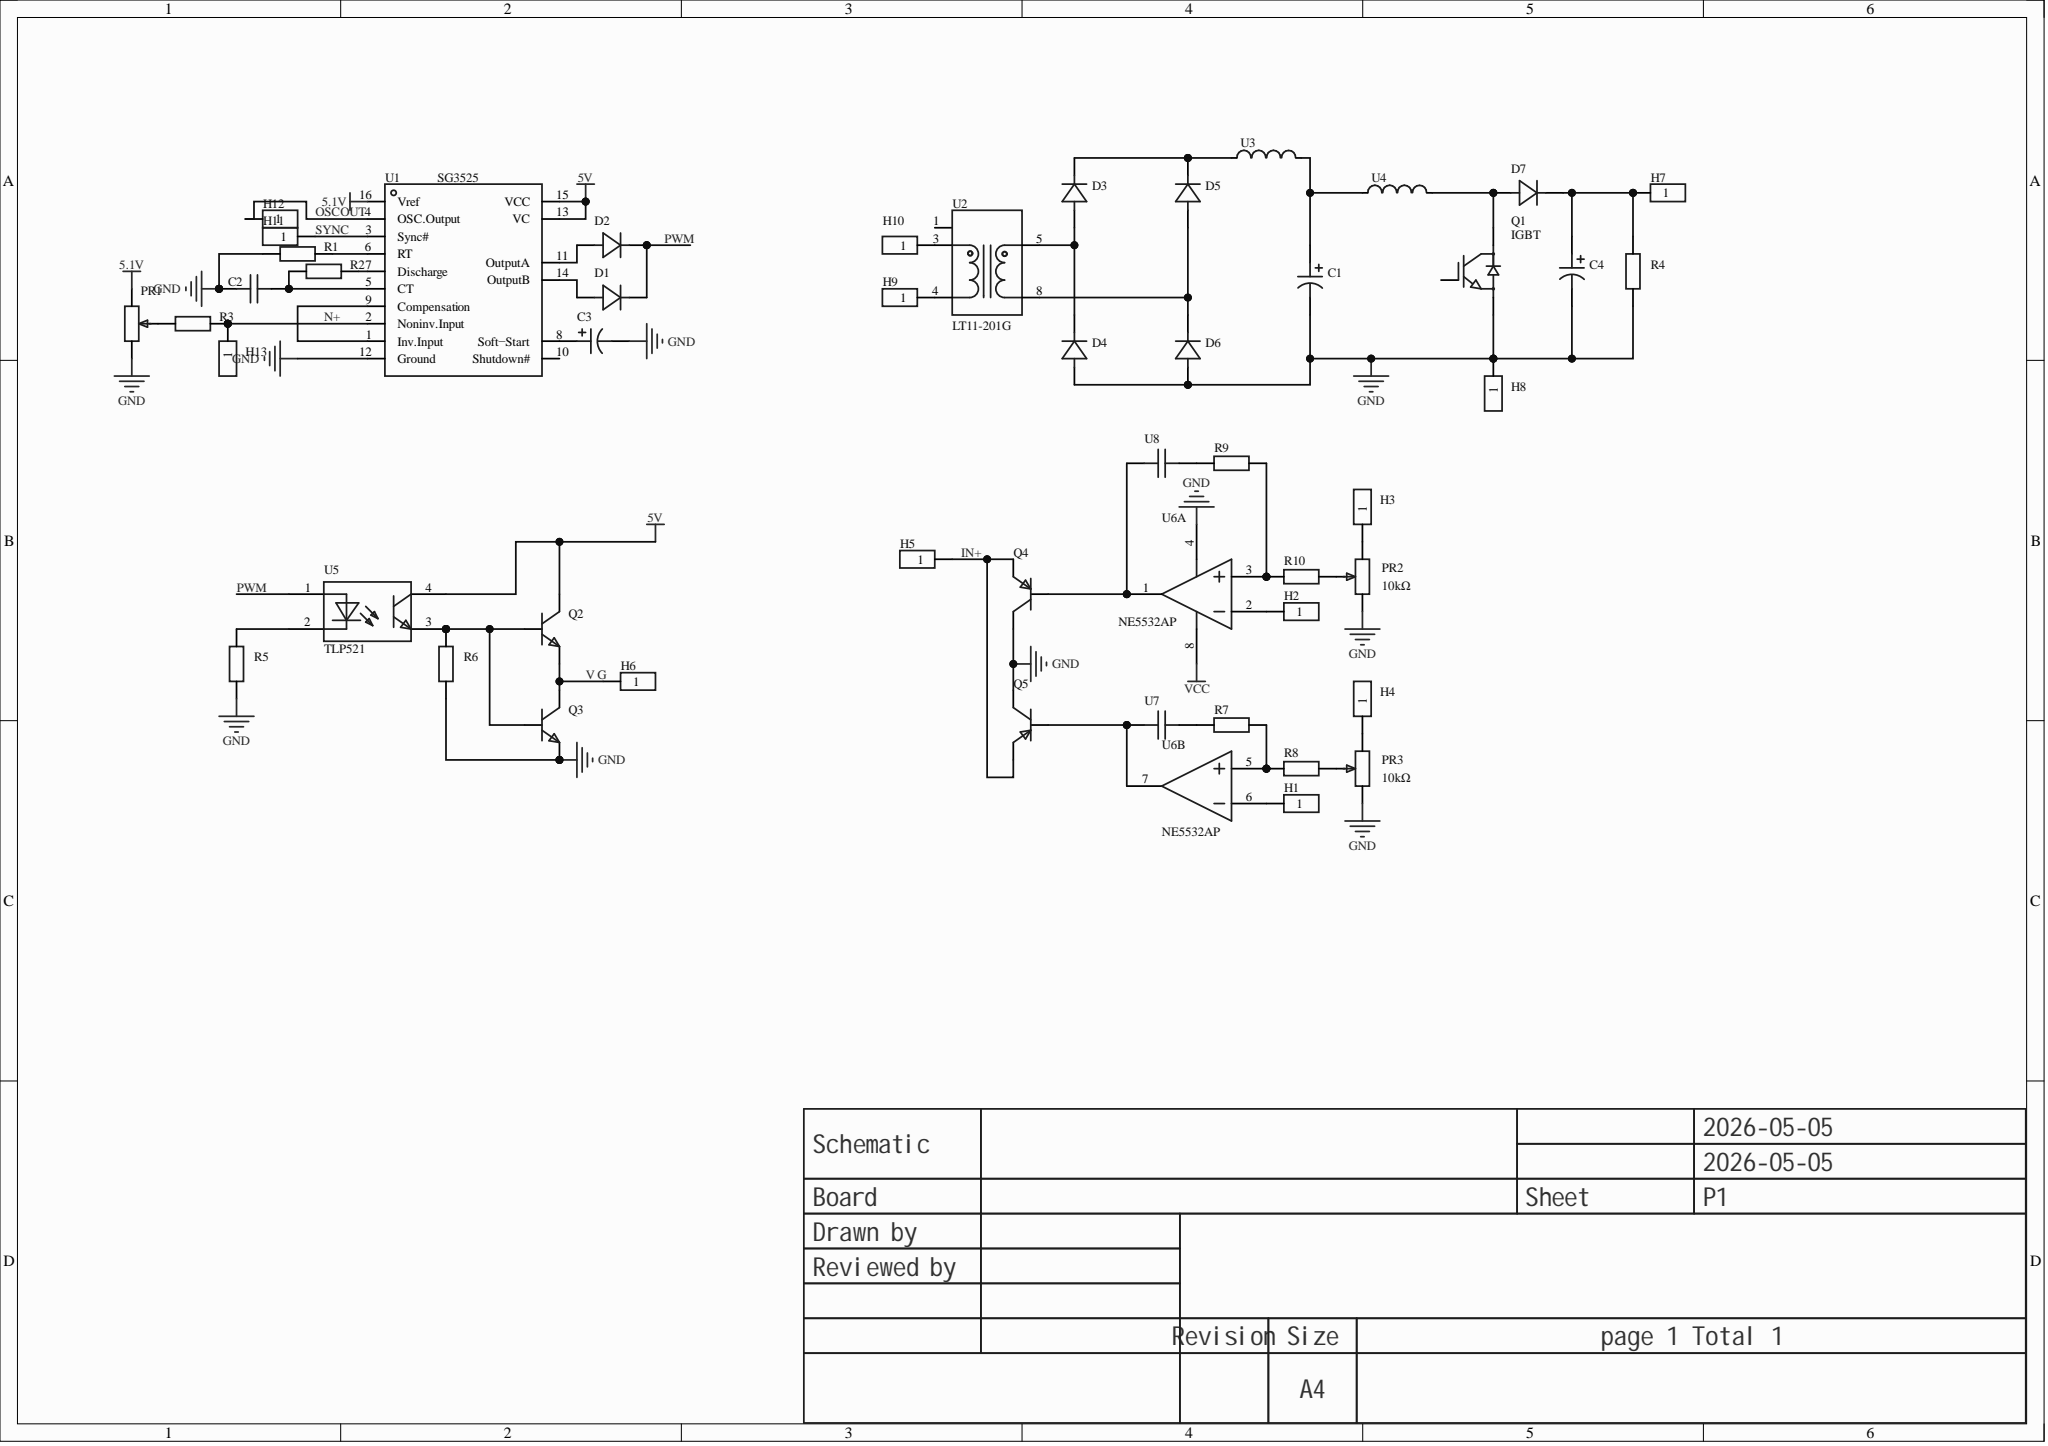Circuit board | Altium Designer | 50 parts | 39 nets
Bill of materials:
Comment,Description,Designator,Footprint,LibRef,Quantity
"10uF","Capacitance:10uF;Tolerance:±20%;Rated voltage:50V;Ripple current:120mA@100KHz;Equivalent series resistance(ESR):1.6Ω;","C1, C3, C4","CAP-TH_BD5.0-P2.00-D0.8-FD-10UF50VC110GL","10UF50VC110GL","3"
"100nF","","C2, U7, U8","CAP-TH_L5.0-W2.5-P5.00-D1.0","100nF","3"
"","","D1, D2, D3, D4, D5, D6, D7","DO_1N4007","D_1N4007A","7"
"","","H1, H2, H3, H4, H5, H6, H7, H8, H9, H10, H11, H12, H13","HDR-TH_1P-V-M_XKB_X4611WV-01I-C28D40","HDR-M_2.54_1x1P","13"
"10kΩ","","PR1, PR2, PR3","R_3296","R_3296","3"
"IGBT","Uses advanced trench gate field-stop technology (Trench FS), collector-emitter breakdown voltage Vces=650V, collector current Ic=40A, with low conduction voltage drop and low turn-off loss, etc…","Q1","TO-247-3_L15.9-W5.0-P5.44-L","MLG40T65FDL-W","1"
"","","Q2, Q3","S8050_TO_92","S8050_TO_NPN","2"
"","","Q4, Q5","S8550P_SOT","S8550_SOT_PNP","2"
"10kΩ","","R1, R2, R3, R4, R5, R6, R7, R8, R9, R10","Res_1/8W","Res_AXIAL-1/8W","10"
"SG3525","Operating voltage: 8V~35V; switching frequency: 100Hz~500kHz; output current: 400mA; transistor withstand voltage: -;","U1","DIP-16_L19.2-W6.6-P2.54-LS7.6-BL","SG3525","1"
"LT11-201G","Transformer  Through-hole broadband carrier coupling transformer, high withstand voltage","U2","XFMR-TH_LT13-201","LT11-201G","1"
"Power inductor (SMD), CKST0502-10uH/M, 10uH, ±20%, 3A, package 5.7mm*5.1mm*2.0mm, Cenke, RoHS","","U3, U4","IND-SMD_L5.7-W5.1","功率电感(贴片),CKST0502-10uH/M,10uH,±20%,3A,封装5.7mm*5.1mm*2.0mm,岑科,RoHS","2"
"TLP521","","U5","SOP-4_L6.4-W4.6-P2.54-LS10.2-TL","TLP521","1"
"NE5532AP","Dual-channel, 30V, 10MHz, low-noise (6nV/vHz) operational amplifier for audio applications","U6","PDIP-8_L9.6-W6.4-P2.54-LS7.6-BL","NE5532AP","1"
Netlist (Protel format):
[
C1
CAP-TH_BD5.0-P2.00-D0.8-FD-10UF50VC110GL
10uF



]
[
C2
CAP-TH_L5.0-W2.5-P5.00-D1.0
100nF



]
[
C3
CAP-TH_BD5.0-P2.00-D0.8-FD-10UF50VC110GL
10uF



]
[
C4
CAP-TH_BD5.0-P2.00-D0.8-FD-10UF50VC110GL
10uF



]
[
D1
DO_1N4007




]
[
D2
DO_1N4007




]
[
D3
DO_1N4007




]
[
D4
DO_1N4007




]
[
D5
DO_1N4007




]
[
D6
DO_1N4007




]
[
D7
DO_1N4007




]
[
H1
HDR-TH_1P-V-M_XKB_X4611WV-01I-C28D40




]
[
H2
HDR-TH_1P-V-M_XKB_X4611WV-01I-C28D40




]
[
H3
HDR-TH_1P-V-M_XKB_X4611WV-01I-C28D40




]
[
H4
HDR-TH_1P-V-M_XKB_X4611WV-01I-C28D40




]
[
H5
HDR-TH_1P-V-M_XKB_X4611WV-01I-C28D40




]
[
H6
HDR-TH_1P-V-M_XKB_X4611WV-01I-C28D40




]
[
H7
HDR-TH_1P-V-M_XKB_X4611WV-01I-C28D40




]
[
H8
HDR-TH_1P-V-M_XKB_X4611WV-01I-C28D40




]
[
H9
HDR-TH_1P-V-M_XKB_X4611WV-01I-C28D40




]
[
H10
HDR-TH_1P-V-M_XKB_X4611WV-01I-C28D40




]
[
H11
HDR-TH_1P-V-M_XKB_X4611WV-01I-C28D40




]
[
H12
HDR-TH_1P-V-M_XKB_X4611WV-01I-C28D40




]
[
H13
HDR-TH_1P-V-M_XKB_X4611WV-01I-C28D40




]
[
PR1
R_3296
10kΩ



]
[
PR2
R_3296
10kΩ



]
[
PR3
R_3296
10kΩ



]
[
Q1
TO-247-3_L15.9-W5.0-P5.44-L
IGBT



]
[
Q2
S8050_TO_92




]
[
Q3
S8050_TO_92




]
[
Q4
S8550P_SOT




]
[
Q5
S8550P_SOT




]
[
R1
Res_1/8W
10kΩ



]
[
R2
Res_1/8W
10kΩ



]
[
R3
Res_1/8W
10kΩ



]
[
R4
Res_1/8W
10kΩ



]
[
R5
Res_1/8W
10kΩ



]
[
R6
Res_1/8W
10kΩ



]
[
R7
Res_1/8W
10kΩ



]
[
R8
Res_1/8W
10kΩ



]
[
R9
Res_1/8W
10kΩ



]
[
R10
Res_1/8W
10kΩ



]
[
U1
DIP-16_L19.2-W6.6-P2.54-LS7.6-BL
SG3525



]
[
U2
XFMR-TH_LT13-201
LT11-201G



]
[
U3
IND-SMD_L5.7-W5.1
Power inductor (SMD), CKST0502-10uH/M, 10uH, ±20%, 3A, package 5.7mm*5.1mm*2.0mm, Cenke, RoHS



]
[
U4
IND-SMD_L5.7-W5.1
Power inductor (SMD), CKST0502-10uH/M, 10uH, ±20%, 3A, package 5.7mm*5.1mm*2.0mm, Cenke, RoHS



]
[
U5
SOP-4_L6.4-W4.6-P2.54-LS10.2-TL
TLP521



]
[
U6
PDIP-8_L9.6-W6.4-P2.54-LS7.6-BL
NE5532AP



]
[
U7
CAP-TH_L5.0-W2.5-P5.00-D1.0
100nF



]
[
U8
CAP-TH_L5.0-W2.5-P5.00-D1.0
100nF



]
(
V G
H6-1
Q2-1
Q3-3
)
(
SYNC
H11-1
U1-3
)
(
PWM
D1-1
D2-1
U5-1
)
(
OSCOUT
H12-1
U1-4
)
(
NetU1_1
U1-1
U1-9
)
(
NetR9_2
R9-2
U8-1
)
(
NetR9_1
R9-1
R10-2
U6-3
)
(
NetR7_2
R7-2
U7-1
)
(
NetR7_1
R7-1
R8-2
U6-5
)
(
NetR5_2
R5-2
U5-2
)
(
NetR2_2
R2-2
U1-7
)
(
NetR1_2
R1-2
U1-6
)
(
NetQ5_1
Q5-1
U6-7
U7-2
)
(
NetQ4_1
Q4-1
U6-1
U8-2
)
(
NetQ2_2
Q2-2
Q3-2
R6-2
U5-3
)
(
NetPR3_2
PR3-2
R8-1
)
(
NetPR2_2
PR2-2
R10-1
)
(
NetPR1_2
PR1-2
R3-1
)
(
NetH10_1
H10-1
U2-3
)
(
NetH9_1
H9-1
U2-4
)
(
NetH4_1
H4-1
PR3-1
)
(
NetH3_1
H3-1
PR2-1
)
(
NetH2_1
H2-1
U6-2
)
(
NetH1_1
H1-1
U6-6
)
(
NetD7_2
D7-2
Q1-2
U4-2
)
(
NetD5_2
D5-2
D6-1
U2-8
)
(
NetD3_2
D3-2
D4-1
U2-5
)
(
NetD3_1
D3-1
D5-1
U3-1
)
(
NetD2_2
D2-2
U1-11
)
(
NetD1_2
D1-2
U1-14
)
(
NetC4_1
C4-1
D7-1
H7-1
R4-2
)
(
NetC3_1
C3-1
U1-8
)
(
NetC2_1
C2-1
R2-1
U1-5
)
(
NetC1_1
C1-1
U3-2
U4-1
)
(
N+
H13-1
R3-2
U1-2
)
(
IN+
H5-1
Q4-2
Q5-2
)
(
GND
C1-2
C2-2
C3-2
C4-2
D4-2
D6-2
H8-1
PR1-1
PR2-3
PR3-3
Q1-3
Q3-1
Q4-3
Q5-3
R1-1
R4-1
R5-1
R6-1
U1-12
U6-4
)
(
5V
Q2-3
U1-13
U1-15
U5-4
)
(
5.1V
PR1-3
U1-16
)